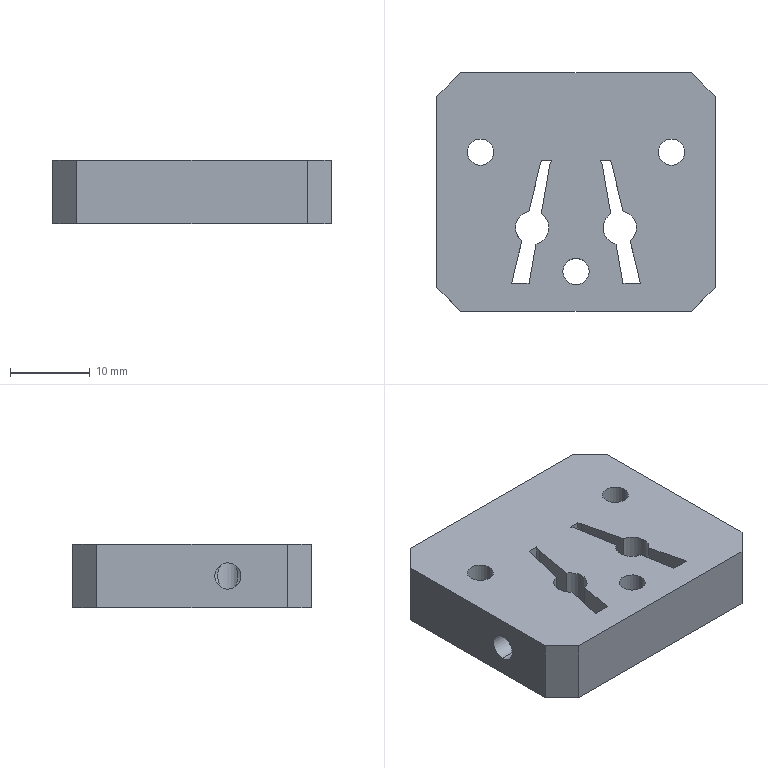Part | STEP file | pin seat 2 | 1 solid | 46 faces | box 35 x 30 x 8 mm | volume 7349 mm3 | plane 22 | cylinder 20 | cone 4 | commonest cylinder face diameters 3.3 x10 4.2 x6 6.8 x2 9.2 x2